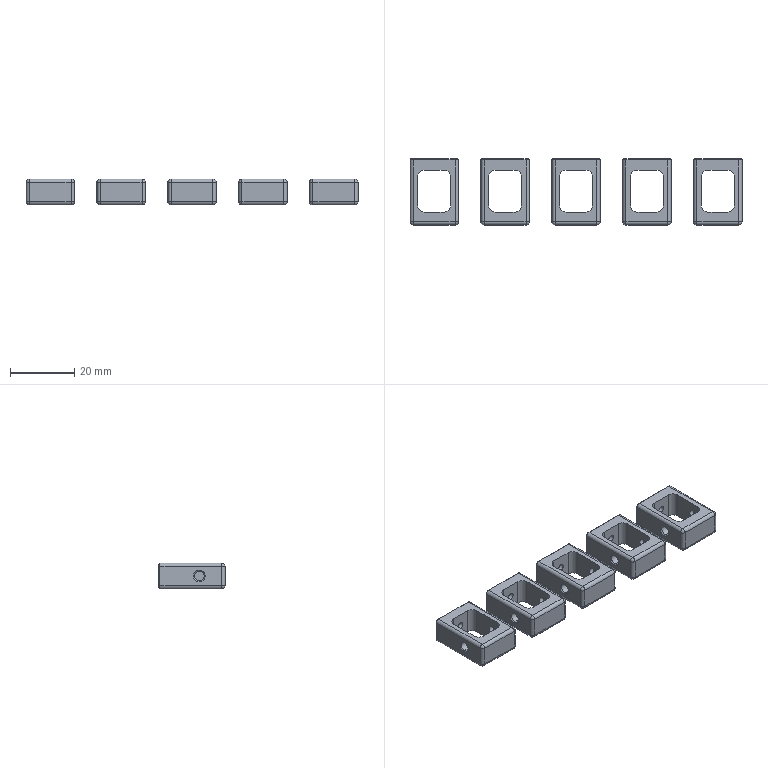NC program | NX | posted with a generic post | part box 103 x 20.5 x 8 mm
Whole program:
N10 G17 G21 G94 G90
(FLOOR_WALL_COPY , TOOL : D80)
N12 T19 M6
N14 G54
N16 G17 G0 G90 X94.5 Y0. S6500 M3
N18 G43 Z30. H19
N20 Z4.
N22 G94 G1 Z1. F1500.
N24 X91.5
N26 X-91.5
N28 X-94.5
N30 Z4.
N32 G0 Z30.
N34 X94.5
N36 Z3.
N38 G1 Z0.
N40 X91.5
N42 X-91.5
N44 X-94.5
N46 Z3.
N48 G0 Z30.
N50 M5
(PLANAR_MILL_COPY_COPY , TOOL : D6A45)
N52 T01 M6
N54 G54
N56 G17 G0 G90 X-47. Y1.02 S9500 M3
N58 G43 Z30. H1
N60 Z0.5
N62 G94 G1 Z-1. F1250.
N64 X-47.7 Y0.616
N66 G3 X-48.2 Y-0.25 R1.
N68 G1 Y-4.75
N70 G3 X-47.1 Y-5.85 R1.1
N72 G1 X-40.9
N74 G3 X-39.8 Y-4.75 R1.1
N76 G1 Y4.25
N78 G3 X-40.9 Y5.35 R1.1
N80 G1 X-47.1
N82 G3 X-48.2 Y4.25 R1.1
N84 G1 Y-0.25
N86 G3 X-47.7 Y-1.116 R1.
N88 G1 X-47. Y-1.52
N90 Z0.5
N92 G0 Z30.
N94 X-25. Y1.02
N96 Z0.5
N98 G1 Z-1.
N100 X-25.7 Y0.616
N102 G3 X-26.2 Y-0.25 R1.
N104 G1 Y-4.75
N106 G3 X-25.1 Y-5.85 R1.1
N108 G1 X-18.9
N110 G3 X-17.8 Y-4.75 R1.1
N112 G1 Y4.25
N114 G3 X-18.9 Y5.35 R1.1
N116 G1 X-25.1
N118 G3 X-26.2 Y4.25 R1.1
N120 G1 Y-0.25
N122 G3 X-25.7 Y-1.116 R1.
N124 G1 X-25. Y-1.52
N126 Z0.5
N128 G0 Z30.
N130 X-3. Y1.02
N132 Z0.5
N134 G1 Z-1.
N136 X-3.7 Y0.616
N138 G3 X-4.2 Y-0.25 R1.
N140 G1 Y-4.75
N142 G3 X-3.1 Y-5.85 R1.1
N144 G1 X3.1
N146 G3 X4.2 Y-4.75 R1.1
N148 G1 Y4.25
N150 G3 X3.1 Y5.35 R1.1
N152 G1 X-3.1
N154 G3 X-4.2 Y4.25 R1.1
N156 G1 Y-0.25
N158 G3 X-3.7 Y-1.116 R1.
N160 G1 X-3. Y-1.52
N162 Z0.5
N164 G0 Z30.
N166 X19. Y1.02
N168 Z0.5
N170 G1 Z-1.
N172 X18.3 Y0.616
N174 G3 X17.8 Y-0.25 R1.
N176 G1 Y-4.75
N178 G3 X18.9 Y-5.85 R1.1
N180 G1 X25.1
N182 G3 X26.2 Y-4.75 R1.1
N184 G1 Y4.25
N186 G3 X25.1 Y5.35 R1.1
N188 G1 X18.9
N190 G3 X17.8 Y4.25 R1.1
N192 G1 Y-0.25
N194 G3 X18.3 Y-1.116 R1.
N196 G1 X19. Y-1.52
N198 Z0.5
N200 G0 Z30.
N202 X47.
N204 Z0.5
N206 G1 Z-1.
N208 X47.7 Y-1.116
N210 G3 X48.2 Y-0.25 R1.
N212 G1 Y4.25
N214 G3 X47.1 Y5.35 R1.1
N216 G1 X40.9
N218 G3 X39.8 Y4.25 R1.1
N220 G1 Y-4.75
N222 G3 X40.9 Y-5.85 R1.1
N224 G1 X47.1
N226 G3 X48.2 Y-4.75 R1.1
N228 G1 Y-0.25
N230 G3 X47.7 Y0.616 R1.
N232 G1 X47. Y1.02
N234 Z0.5
N236 G0 Z30.
N238 M5
(ZLEVEL_PROFILE_1_COPY , TOOL : D4R0.5)
N240 T16 M6
N242 G54
N244 G17 G0 G90 X35.175 Y-12.738 S9500 M3
N246 G43 Z30. H16
N248 Z1.488
N250 G94 G1 Z-0.012 F3000.
N252 X35.682 Y-12.485
N254 G3 X35.903 Y-12.152 R0.4
N256 X35.813 Y-9.95 R10.813
N258 G1 Y9.25
N260 G2 X37.5 Y10.937 R1.687
N262 G1 X50.5
N264 G2 X52.187 Y9.25 R1.687
N266 G1 Y-9.95
N268 X52.109 Y-10.153
N270 X52.09 Y-12.155
N272 X52.133 Y-12.154 Z-0.018
N274 X52.161 Y-12.153 Z-0.024
N276 X52.25 Y-10.153
N278 X52.27 Y-9.95
N280 Y9.25
N282 G3 X50.5 Y11.02 R1.77
N284 G1 X37.5
N286 G3 X35.73 Y9.25 R1.77
N288 G1 Y-9.95
N290 G2 X35.826 Y-12.151 R9.258
N292 G1 X35.785 Y-12.152 Z-0.032
N294 X35.752 Y-12.153 Z-0.039
N296 G3 X35.66 Y-9.95 R7.979
N298 G1 Y9.25
N300 G2 X37.5 Y11.09 R1.84
N302 G1 X50.5
N304 G2 X52.34 Y9.25 R1.84
N306 G1 Y-9.95
N308 X52.223 Y-12.151
N310 X52.264 Y-12.15 Z-0.049
N312 X52.289 Z-0.058
N314 X52.299 Y-11.846
N316 X52.414 Y-9.95
N318 Y9.25
N320 G3 X50.5 Y11.164 R1.914
N322 G1 X37.5
N324 G3 X35.586 Y9.25 R1.914
N326 G1 Y-9.95
N328 G2 X35.684 Y-12.151 R9.178
N330 G1 X35.643 Z-0.07
N332 X35.606 Y-12.15 Z-0.083
N334 G3 X35.509 Y-9.95 R11.176
N336 G1 Y9.25
N338 G2 X37.5 Y11.241 R1.991
N340 G1 X50.5
N342 G2 X52.491 Y9.25 R1.991
N344 G1 Y-9.95
N346 X52.473 Y-10.153
N348 X52.354 Y-12.15
N350 X52.406 Z-0.097
N352 X52.431 Z-0.112
N354 G2 X52.568 Y-9.95 R21.926
N356 G1 Y9.25
N358 G3 X50.5 Y11.318 R2.068
N360 G1 X37.5
N362 G3 X35.432 Y9.25 R2.068
N364 G1 Y-9.95
N366 G2 X35.539 Y-12.15 R11.662
N368 G1 X35.494 Z-0.129
N370 X35.463 Z-0.146
N372 G3 X35.355 Y-9.95 R12.693
N374 G1 Y9.25
N376 G2 X37.5 Y11.395 R2.145
N378 G1 X50.5
N380 G2 X52.645 Y9.25 R2.145
N382 G1 Y-9.95
N384 G3 X52.522 Y-12.15 R18.767
N386 G1 X52.574 Z-0.166
N388 X52.621 Y-12.151 Z-0.186
N390 G2 X52.724 Y-9.95 R19.723
N392 G1 Y9.25
N394 G3 X50.5 Y11.474 R2.224
N396 G1 X37.5
N398 G3 X35.276 Y9.25 R2.224
N400 G1 Y-9.95
N402 G2 X35.374 Y-12.15 R17.072
N404 G1 X35.323 Z-0.21
N406 X35.286 Z-0.233
N408 G3 X35.197 Y-9.95 R17.343
N410 G1 Y9.25
N412 G2 X37.5 Y11.553 R2.303
N414 G1 X50.5
N416 G2 X52.803 Y9.25 R2.303
N418 G1 Y-9.95
N420 G3 X52.716 Y-12.151 R17.692
N422 G1 X52.761 Z-0.259
N424 X52.796 Y-12.15 Z-0.286
N426 G2 X52.881 Y-9.95 R18.852
N428 G1 Y9.25
N430 G3 X50.5 Y11.631 R2.381
N432 G1 X37.5
N434 G3 X35.119 Y9.25 R2.381
N436 G1 Y-9.95
N438 G2 X35.212 Y-12.15 R17.769
N440 G1 X35.16 Z-0.315
N442 X35.13 Z-0.344
N444 G3 X35.044 Y-9.95 R18.76
N446 G1 Y9.25
N448 G2 X37.5 Y11.706 R2.456
N450 G1 X50.5
N452 G2 X52.956 Y9.25 R2.456
N454 G1 Y-9.95
N456 G3 X52.877 Y-12.15 R19.225
N458 G1 X52.92 Y-12.151 Z-0.376
N460 X52.96 Z-0.408
N462 G2 X53.028 Y-9.95 R23.684
N464 G1 Y9.25
N466 G3 X50.5 Y11.778 R2.528
N468 G1 X37.5
N470 G3 X34.972 Y9.25 R2.528
N472 G1 Y-9.95
N474 G2 X35.04 Y-12.15 R23.709
N476 G1 X34.995 Y-12.151 Z-0.443
N478 X34.96 Z-0.477
N480 G3 X34.903 Y-9.95 R26.088
N482 G1 Y9.25
N484 G2 X37.5 Y11.847 R2.597
N486 G1 X50.5
N488 G2 X53.097 Y9.25 R2.597
N490 G1 Y-9.95
N492 G3 X53.04 Y-12.152 R27.115
N494 G1 X53.073 Y-12.151 Z-0.514
N496 X53.1 Y-12.15 Z-0.551
N498 G2 X53.162 Y-9.95 R24.243
N500 G1 Y9.25
N502 G3 X50.5 Y11.912 R2.662
N504 G1 X37.5
N506 G3 X34.838 Y9.25 R2.662
N508 G1 Y-9.95
N510 G2 X34.9 Y-12.151 R24.274
N512 G1 X34.868 Z-0.59
N514 X34.841 Z-0.629
N516 G3 X34.779 Y-9.95 R24.293
N518 G1 Y9.25
N520 G2 X37.5 Y11.971 R2.721
N522 G1 X50.5
N524 G2 X53.221 Y9.25 R2.721
N526 G1 Y-9.95
N528 G3 X53.159 Y-12.151 R24.303
N530 G1 X53.193 Z-0.67
N532 X53.221 Y-12.152 Z-0.711
N534 G2 X53.276 Y-9.95 R30.814
N536 G1 Y9.25
N538 G3 X50.5 Y12.026 R2.776
N540 G1 X37.5
N542 G3 X34.724 Y9.25 R2.776
N544 G1 Y-9.95
N546 G2 X34.779 Y-12.15 R30.37
N548 G1 X34.746 Y-12.151 Z-0.754
N550 X34.728 Z-0.797
N552 G3 X34.675 Y-9.95 R31.84
N554 G1 Y9.25
N556 G2 X37.5 Y12.075 R2.825
N558 G1 X50.5
N560 G2 X53.325 Y9.25 R2.825
N562 G1 Y-9.95
N564 G3 X53.274 Y-12.151 R28.165
N566 G1 X53.299 Z-0.842
N568 X53.317 Z-0.887
N570 G2 X53.369 Y-9.95 R25.497
N572 G1 Y9.25
N574 G3 X50.5 Y12.119 R2.869
N576 G1 X37.5
N578 G3 X34.631 Y9.25 R2.869
N580 G1 Y-9.95
N582 G2 X34.688 Y-12.153 R33.716
N584 G1 X34.663 Y-12.155 Z-0.933
N586 X34.647 Y-12.156 Z-0.979
N588 G3 X34.593 Y-9.95 R49.451
N590 G1 Y9.25
N592 G2 X37.5 Y12.157 R2.907
N594 G1 X50.5
N596 G2 X53.407 Y9.25 R2.907
N598 G1 Y-9.95
N600 G3 X53.362 Y-12.15 R27.233
N602 G1 X53.384 Z-1.026
N604 X53.403 Z-1.074
N606 G2 X53.438 Y-9.95 R31.796
N608 G1 Y9.25
N610 G3 X50.5 Y12.188 R2.938
N612 G1 X37.5
N614 G3 X34.562 Y9.25 R2.938
N616 G1 Y-9.95
N618 G2 X34.608 Y-12.158 R55.585
N620 G1 X34.589 Y-12.16 Z-1.122
N622 X34.572 Y-12.161 Z-1.17
N624 G3 X34.537 Y-9.95 R85.134
N626 G1 Y9.25
N628 G2 X37.5 Y12.213 R2.963
N630 G1 X50.5
N632 G2 X53.463 Y9.25 R2.963
N634 G1 Y-9.95
N636 G3 X53.436 Y-12.152 R39.114
N638 G1 X53.446 Y-12.153 Z-1.212
N640 X53.456 Z-1.253
N642 X53.458 Y-10.717
N644 X53.469 Y-10.435
N646 G2 X53.479 Y-9.95 R3.288
N648 G1 Y9.25
N650 G3 X50.5 Y12.229 R2.979
N652 G1 X37.5
N654 G3 X34.521 Y9.25 R2.979
N656 G1 Y-9.95
N658 G2 X34.55 Y-12.162 R76.351
N660 G1 X34.538 Y-12.163 Z-1.294
N662 X34.531 Z-1.335
N664 X34.516 Y-10.153
N666 X34.509 Y-9.95
N668 Y9.25
N670 G2 X37.5 Y12.241 R2.991
N672 G1 X50.5
N674 G2 X53.491 Y9.25 R2.991
N676 G1 Y-9.95
N678 G3 X53.475 Y-10.717 R24.677
N680 G1 X53.473 Y-12.154
N682 X53.483 Y-12.155 Z-1.376
N684 X53.49 Y-12.156 Z-1.418
N686 X53.492 Y-12.128
N688 X53.496 Y9.273
N690 G3 X53.48 Y9.577 R2.784
N692 X51.216 Y12.161 R2.998
N694 X50.51 Y12.248 R2.956
N696 G1 X37.5
N698 G3 X34.502 Y9.25 R2.998
N700 G1 Y-9.95
N702 X34.511 Y-12.165
N704 X34.505 Y-12.162 Z-1.5
N706 X34.5 Y9.247
N708 G2 X35.313 Y11.3 R2.999
N710 X36.133 Y11.918 R2.897
N712 X36.711 Y12.14 R3.11
N714 X37.518 Y12.248 R3.053
N716 G1 X50.507
N718 G2 X51.524 Y12.069 R2.963
N720 X53.322 Y10.265 R3.012
N722 X53.498 Y9.266 R2.931
N724 G1 X53.495 Y-12.155
N726 G3 X53.695 Y-12.502 R0.4
N728 G1 X54.218 Y-12.804
N730 Z0.
N732 G0 Z3.
N734 X13.176 Y-12.751
N736 Z1.488
N738 G1 Z-0.012
N740 X13.687 Y-12.489
N742 G3 X13.905 Y-12.153 R0.4
N744 X13.813 Y-9.95 R11.978
N746 G1 Y9.25
N748 G2 X15.5 Y10.937 R1.687
N750 G1 X28.5
N752 G2 X30.187 Y9.25 R1.687
N754 G1 Y-9.95
N756 X30.114 Y-10.153
N758 X30.103 Y-12.155
N760 X30.16 Y-12.153 Z-0.024
N762 X30.17 Y-11.846
N764 X30.27 Y-9.95
N766 Y9.25
N768 G3 X28.5 Y11.02 R1.77
N770 G1 X15.5
N772 G3 X13.73 Y9.25 R1.77
N774 G1 Y-9.95
N776 G2 X13.828 Y-12.15 R10.515
N778 G1 X13.781 Z-0.032
N780 X13.776 Z-0.039
N782 G3 X13.66 Y-9.95 R9.336
N784 G1 Y9.25
N786 G2 X15.5 Y11.09 R1.84
N788 G1 X28.5
N790 G2 X30.34 Y9.25 R1.84
N792 G1 Y-9.95
N794 G3 X30.226 Y-12.15 R18.109
N796 G1 X30.26 Z-0.049
N798 X30.281 Z-0.058
N800 G2 X30.414 Y-9.95 R19.419
N802 G1 Y9.25
N804 G3 X28.5 Y11.164 R1.914
N806 G1 X15.5
N808 G3 X13.586 Y9.25 R1.914
N810 G1 Y-9.95
N812 G2 X13.706 Y-12.15 R9.374
N814 G1 X13.643 Z-0.07
N816 X13.618 Z-0.083
N818 G3 X13.509 Y-9.95 R10.828
N820 G1 Y9.25
N822 G2 X15.5 Y11.241 R1.991
N824 G1 X28.5
N826 G2 X30.491 Y9.25 R1.991
N828 G1 Y-9.95
N830 G3 X30.349 Y-12.15 R18.798
N832 G1 X30.406 Z-0.097
N834 X30.431 Z-0.112
N836 G2 X30.568 Y-9.95 R19.096
N838 G1 Y9.25
N840 G3 X28.5 Y11.318 R2.068
N842 G1 X15.5
N844 G3 X13.432 Y9.25 R2.068
N846 G1 Y-9.95
N848 G2 X13.533 Y-12.15 R11.751
N850 G1 X13.494 Z-0.129
N852 X13.46 Z-0.146
N854 G3 X13.355 Y-9.95 R12.417
N856 G1 Y9.25
N858 G2 X15.5 Y11.395 R2.145
N860 G1 X28.5
N862 G2 X30.645 Y9.25 R2.145
N864 G1 Y-9.95
N866 G3 X30.525 Y-12.15 R18.309
N868 G1 X30.574 Y-12.151 Z-0.166
N870 X30.621 Z-0.186
N872 G2 X30.724 Y-9.95 R18.599
N874 G1 Y9.25
N876 G3 X28.5 Y11.474 R2.224
N878 G1 X15.5
N880 G3 X13.276 Y9.25 R2.224
N882 G1 Y-9.95
N884 G2 X13.375 Y-12.15 R15.774
N886 G1 X13.324 Z-0.21
N888 X13.276 Z-0.233
N890 G3 X13.197 Y-9.95 R18.579
N892 G1 Y9.25
N894 G2 X15.5 Y11.553 R2.303
N896 G1 X28.5
N898 G2 X30.803 Y9.25 R2.303
N900 G1 Y-9.95
N902 G3 X30.711 Y-12.151 R19.024
N904 G1 X30.767 Y-12.15 Z-0.259
N906 X30.801 Z-0.286
N908 G2 X30.881 Y-9.95 R18.564
N910 G1 Y9.25
N912 G3 X28.5 Y11.631 R2.381
N914 G1 X15.5
N916 G3 X13.119 Y9.25 R2.381
N918 G1 Y-9.95
N920 G2 X13.206 Y-12.15 R16.93
N922 G1 X13.159 Z-0.315
N924 X13.128 Z-0.344
N926 G3 X13.044 Y-9.95 R17.802
N928 G1 Y9.25
N930 G2 X15.5 Y11.706 R2.456
N932 G1 X28.5
N934 G2 X30.956 Y9.25 R2.456
N936 G1 Y-9.95
N938 G3 X30.877 Y-12.15 R17.906
N940 G1 X30.92 Y-12.151 Z-0.376
N942 X30.96 Z-0.408
N944 G2 X31.028 Y-9.95 R19.425
N946 G1 Y9.25
N948 G3 X28.5 Y11.778 R2.528
N950 G1 X15.5
N952 G3 X12.972 Y9.25 R2.528
N954 G1 Y-9.95
N956 G2 X13.042 Y-12.15 R23.333
N958 G1 X12.995 Z-0.443
N960 X12.967 Z-0.477
N962 G3 X12.903 Y-9.95 R24.397
N964 G1 Y9.25
N966 G2 X15.5 Y11.847 R2.597
N968 G1 X28.5
N970 G2 X31.097 Y9.25 R2.597
N972 G1 Y-9.95
N974 G3 X31.037 Y-12.15 R22.861
N976 G1 X31.069 Z-0.514
N978 X31.1 Z-0.551
N980 G2 X31.162 Y-9.95 R24.207
N982 G1 Y9.25
N984 G3 X28.5 Y11.912 R2.662
N986 G1 X15.5
N988 G3 X12.838 Y9.25 R2.662
N990 G1 Y-9.95
N992 G2 X12.904 Y-12.15 R23.42
N994 G1 X12.868 Y-12.151 Z-0.59
N996 X12.841 Z-0.629
N998 G3 X12.779 Y-9.95 R23.43
N1000 G1 Y9.25
N1002 G2 X15.5 Y11.971 R2.721
N1004 G1 X28.5
N1006 G2 X31.221 Y9.25 R2.721
N1008 G1 Y-9.95
N1010 G3 X31.16 Y-12.151 R24.729
N1012 G1 X31.193 Z-0.67
N1014 X31.222 Z-0.711
N1016 G2 X31.276 Y-9.95 R29.092
N1018 G1 Y9.25
N1020 G3 X28.5 Y12.026 R2.776
N1022 G1 X15.5
N1024 G3 X12.724 Y9.25 R2.776
N1026 G1 Y-9.95
N1028 G2 X12.784 Y-12.15 R25.622
N1030 G1 X12.745 Z-0.754
N1032 X12.726 Z-0.797
N1034 G3 X12.675 Y-9.95 R32.986
N1036 G1 Y9.25
N1038 G2 X15.5 Y12.075 R2.825
N1040 G1 X28.5
N1042 G2 X31.325 Y9.25 R2.825
N1044 G1 Y-9.95
N1046 G3 X31.275 Y-12.152 R33.248
N1048 G1 X31.299 Y-12.151 Z-0.842
N1050 X31.319 Z-0.887
N1052 G2 X31.369 Y-9.95 R28.16
N1054 G1 Y9.25
N1056 G3 X28.5 Y12.119 R2.869
N1058 G1 X15.5
N1060 G3 X12.631 Y9.25 R2.869
N1062 G1 Y-9.95
N1064 G2 X12.684 Y-12.152 R32.786
N1066 G1 X12.663 Y-12.153 Z-0.933
N1068 X12.645 Y-12.154 Z-0.979
N1070 G3 X12.593 Y-9.95 R43.797
N1072 G1 Y9.25
N1074 G2 X15.5 Y12.157 R2.907
N1076 G1 X28.5
N1078 G2 X31.407 Y9.25 R2.907
N1080 G1 Y-9.95
N1082 G3 X31.363 Y-12.15 R27.185
N1084 G1 X31.386 Y-12.152 Z-1.026
N1086 X31.401 Y-12.153 Z-1.074
N1088 G2 X31.438 Y-9.95 R32.305
N1090 G1 Y9.25
N1092 G3 X28.5 Y12.188 R2.938
N1094 G1 X15.5
N1096 G3 X12.562 Y9.25 R2.938
N1098 G1 Y-9.95
N1100 G2 X12.606 Y-12.157 R59.474
N1102 G1 X12.589 Y-12.158 Z-1.122
N1104 X12.572 Y-12.159 Z-1.17
N1106 G3 X12.537 Y-9.95 R87.828
N1108 G1 Y9.25
N1110 G2 X15.5 Y12.213 R2.963
N1112 G1 X28.5
N1114 G2 X31.463 Y9.25 R2.963
N1116 G1 Y-9.95
N1118 G3 X31.436 Y-12.155 R40.13
N1120 G1 X31.446 Z-1.212
N1122 X31.461 Y-12.156 Z-1.253
N1124 G2 X31.479 Y-9.95 R52.452
N1126 G1 Y9.25
N1128 G3 X28.5 Y12.229 R2.979
N1130 G1 X15.5
N1132 G3 X12.521 Y9.25 R2.979
N1134 G1 Y-9.95
N1136 G2 X12.548 Y-12.159 R75.91
N1138 G1 X12.538 Y-12.16 Z-1.294
N1140 X12.53 Y-12.161 Z-1.335
N1142 X12.516 Y-10.153
N1144 X12.509 Y-9.95
N1146 Y9.25
N1148 G2 X15.5 Y12.241 R2.991
N1150 G1 X28.5
N1152 G2 X31.491 Y9.25 R2.991
N1154 G1 Y-9.95
N1156 G3 X31.476 Y-12.157 R76.85
N1158 G1 X31.48 Z-1.376
N1160 X31.491 Y-12.158 Z-1.418
N1162 X31.494 Y-10.153
N1164 X31.497 Y9.272
N1166 G3 X31.48 Y9.574 R2.791
N1168 X29.946 Y11.876 R2.998
N1170 G1 X29.717 Y11.99
N1172 G3 X29.082 Y12.191 R2.998
N1174 X28.5 Y12.248 R2.998
N1176 G1 X15.471
N1178 G3 X13.606 Y11.574 R2.998
N1180 G1 X13.402 Y11.391
N1182 G3 X12.502 Y9.25 R2.998
N1184 G1 Y-9.95
N1186 X12.511 Y-12.162
N1188 X12.505 Y-12.16 Z-1.5
N1190 X12.5 Y9.247
N1192 G2 X13.605 Y11.572 R2.999
N1194 X14.078 Y11.889 R2.738
N1196 X15.35 Y12.242 R2.945
N1198 G1 X15.49 Y12.248
N1200 X28.5
N1202 G2 X29.496 Y12.076 R2.942
N1204 G1 X29.761 Y11.972
N1206 G2 X31.133 Y10.683 R3.033
N1208 X31.498 Y9.26 R3.007
N1210 G1 X31.496 Y-12.128
N1212 X31.495 Y-12.157
N1214 G3 X31.676 Y-12.514 R0.4
N1216 G1 X32.206 Y-12.859
N1218 Z0.
N1220 G0 Z3.
N1222 X-8.825 Y-12.741
N1224 Z1.488
N1226 G1 Z-0.012
N1228 X-8.323 Y-12.489
N1230 G3 X-8.103 Y-12.154 R0.4
N1232 X-8.187 Y-9.95 R11.509
N1234 G1 Y9.25
N1236 G2 X-6.5 Y10.937 R1.687
N1238 G1 X6.5
N1240 G2 X8.187 Y9.25 R1.687
N1242 G1 Y-9.95
N1244 X8.168 Y-10.153
N1246 X8.095 Y-12.155
N1248 X8.134 Y-12.153 Z-0.018
N1250 X8.159 Y-12.152 Z-0.024
N1252 X8.237 Y-10.153
N1254 X8.27 Y-9.95
N1256 Y9.25
N1258 G3 X6.5 Y11.02 R1.77
N1260 G1 X-6.5
N1262 G3 X-8.27 Y9.25 R1.77
N1264 G1 Y-9.95
N1266 G2 X-8.179 Y-12.151 R11.718
N1268 G1 X-8.221 Y-12.15 Z-0.032
N1270 X-8.232 Z-0.039
N1272 G3 X-8.34 Y-9.95 R10.746
N1274 G1 Y9.25
N1276 G2 X-6.5 Y11.09 R1.84
N1278 G1 X6.5
N1280 G2 X8.34 Y9.25 R1.84
N1282 G1 Y-9.95
N1284 X8.298 Y-10.153
N1286 X8.216 Y-12.15
N1288 X8.26 Z-0.049
N1290 X8.274 Z-0.058
N1292 X8.285 Y-11.846
N1294 X8.378 Y-10.153
N1296 X8.414 Y-9.95
N1298 Y9.25
N1300 G3 X6.5 Y11.164 R1.914
N1302 G1 X-6.5
N1304 G3 X-8.414 Y9.25 R1.914
N1306 G1 Y-9.95
N1308 G2 X-8.294 Y-12.15 R9.95
N1310 G1 X-8.357 Z-0.07
N1312 X-8.372 Z-0.083
N1314 G3 X-8.491 Y-9.95 R10.072
N1316 G1 Y9.25
N1318 G2 X-6.5 Y11.241 R1.991
N1320 G1 X6.5
N1322 G2 X8.491 Y9.25 R1.991
N1324 G1 Y-9.95
N1326 G3 X8.348 Y-12.15 R19.167
N1328 G1 X8.405 Z-0.097
N1330 X8.435 Z-0.112
N1332 G2 X8.568 Y-9.95 R20.551
N1334 G1 Y9.25
N1336 G3 X6.5 Y11.318 R2.068
N1338 G1 X-6.5
N1340 G3 X-8.568 Y9.25 R2.068
N1342 G1 Y-9.95
N1344 G2 X-8.465 Y-12.15 R10.922
N1346 G1 X-8.506 Z-0.129
N1348 X-8.538 Z-0.146
N1350 G3 X-8.645 Y-9.95 R11.832
N1352 G1 Y9.25
N1354 G2 X-6.5 Y11.395 R2.145
N1356 G1 X6.5
N1358 G2 X8.645 Y9.25 R2.145
N1360 G1 Y-9.95
N1362 G3 X8.521 Y-12.15 R16.287
N1364 G1 X8.574 Z-0.166
N1366 X8.61 Z-0.186
N1368 G2 X8.724 Y-9.95 R17.188
N1370 G1 Y9.25
N1372 G3 X6.5 Y11.474 R2.224
N1374 G1 X-6.5
N1376 G3 X-8.724 Y9.25 R2.224
N1378 G1 Y-9.95
N1380 G2 X-8.621 Y-12.15 R13.891
N1382 G1 X-8.677 Z-0.21
N1384 X-8.716 Z-0.233
N1386 G3 X-8.803 Y-9.95 R20.219
N1388 G1 Y9.25
N1390 G2 X-6.5 Y11.553 R2.303
N1392 G1 X6.5
N1394 G2 X8.803 Y9.25 R2.303
N1396 G1 Y-9.95
N1398 G3 X8.712 Y-12.15 R22.154
N1400 G1 X8.76 Z-0.259
N1402 X8.798 Z-0.286
N1404 G2 X8.881 Y-9.95 R17.875
N1406 G1 Y9.25
N1408 G3 X6.5 Y11.631 R2.381
N1410 G1 X-6.5
N1412 G3 X-8.881 Y9.25 R2.381
N1414 G1 Y-9.95
N1416 G2 X-8.798 Y-12.15 R17.875
N1418 G1 X-8.841 Z-0.315
N1420 X-8.872 Z-0.344
N1422 G3 X-8.956 Y-9.95 R17.78
N1424 G1 Y9.25
N1426 G2 X-6.5 Y11.706 R2.456
N1428 G1 X6.5
N1430 G2 X8.956 Y9.25 R2.456
N1432 G1 Y-9.95
N1434 G3 X8.872 Y-12.15 R17.78
N1436 G1 X8.92 Z-0.376
N1438 X8.953 Z-0.408
N1440 G2 X9.028 Y-9.95 R21.292
N1442 G1 Y9.25
N1444 G3 X6.5 Y11.778 R2.528
N1446 G1 X-6.5
N1448 G3 X-9.028 Y9.25 R2.528
N1450 G1 Y-9.95
N1452 G2 X-8.953 Y-12.15 R21.292
N1454 G1 X-8.998 Z-0.443
N1456 X-9.041 Z-0.477
N1458 G3 X-9.097 Y-9.95 R25.737
N1460 G1 Y9.25
N1462 G2 X-6.5 Y11.847 R2.597
N1464 G1 X6.5
N1466 G2 X9.097 Y9.25 R2.597
N1468 G1 Y-9.95
N1470 G3 X9.041 Y-12.15 R25.737
N1472 G1 X9.073 Z-0.514
N1474 X9.098 Z-0.551
N1476 G2 X9.162 Y-9.95 R23.081
N1478 G1 Y9.25
N1480 G3 X6.5 Y11.912 R2.662
N1482 G1 X-6.5
N1484 G3 X-9.162 Y9.25 R2.662
N1486 G1 Y-9.95
N1488 G2 X-9.098 Y-12.15 R23.084
N1490 G1 X-9.132 Y-12.151 Z-0.59
N1492 X-9.16 Z-0.629
N1494 G3 X-9.221 Y-9.95 R24.413
N1496 G1 Y9.25
N1498 G2 X-6.5 Y11.971 R2.721
N1500 G1 X6.5
N1502 G2 X9.221 Y9.25 R2.721
N1504 G1 Y-9.95
N1506 G3 X9.16 Y-12.151 R24.402
N1508 G1 X9.193 Z-0.67
N1510 X9.222 Z-0.711
N1512 G2 X9.276 Y-9.95 R30.188
N1514 G1 Y9.25
N1516 G3 X6.5 Y12.026 R2.776
N1518 G1 X-6.5
N1520 G3 X-9.276 Y9.25 R2.776
N1522 G1 Y-9.95
N1524 G2 X-9.222 Y-12.152 R30.24
N1526 G1 X-9.249 Y-12.151 Z-0.754
N1528 X-9.273 Z-0.797
N1530 G3 X-9.325 Y-9.95 R32.017
N1532 G1 Y9.25
N1534 G2 X-6.5 Y12.075 R2.825
N1536 G1 X6.5
N1538 G2 X9.325 Y9.25 R2.825
N1540 G1 Y-9.95
N1542 G3 X9.275 Y-12.151 R29.563
N1544 G1 X9.3 Y-12.15 Z-0.842
N1546 X9.32 Z-0.887
N1548 G2 X9.369 Y-9.95 R27.833
N1550 G1 Y9.25
N1552 G3 X6.5 Y12.119 R2.869
N1554 G1 X-6.5
N1556 G3 X-9.369 Y9.25 R2.869
N1558 G1 Y-9.95
N1560 G2 X-9.316 Y-12.15 R33.813
N1562 G1 X-9.337 Y-12.151 Z-0.933
N1564 X-9.354 Y-12.152 Z-0.979
N1566 G3 X-9.407 Y-9.95 R41.05
N1568 G1 Y9.25
N1570 G2 X-6.5 Y12.157 R2.907
N1572 G1 X6.5
N1574 G2 X9.407 Y9.25 R2.907
N1576 G1 Y-9.95
N1578 G3 X9.362 Y-12.152 R27.311
N1580 G1 X9.383 Y-12.154 Z-1.026
N1582 X9.405 Y-12.156 Z-1.074
N1584 G2 X9.438 Y-9.95 R32.12
N1586 G1 Y9.25
N1588 G3 X6.5 Y12.188 R2.938
N1590 G1 X-6.5
N1592 G3 X-9.438 Y9.25 R2.938
N1594 G1 Y-9.95
N1596 G2 X-9.393 Y-12.155 R76.635
N1598 G1 X-9.411 Y-12.156 Z-1.122
N1600 X-9.428 Y-12.157 Z-1.17
N1602 G3 X-9.463 Y-9.95 R98.832
N1604 G1 Y9.25
N1606 G2 X-6.5 Y12.213 R2.963
N1608 G1 X6.5
N1610 G2 X9.463 Y9.25 R2.963
N1612 G1 Y-9.95
N1614 G3 X9.436 Y-12.157 R39.697
N1616 G1 X9.446 Z-1.212
N1618 X9.458 Z-1.253
N1620 X9.457 Y-11.846
N1622 X9.468 Y-10.153
N1624 X9.479 Y-9.95
N1626 Y9.25
N1628 G3 X6.5 Y12.229 R2.979
N1630 G1 X-6.5
N1632 G3 X-9.479 Y9.25 R2.979
N1634 G1 Y-9.95
N1636 X-9.47 Y-10.153
N1638 X-9.454 Y-12.158
N1640 X-9.462 Y-12.159 Z-1.294
N1642 X-9.472 Z-1.335
N1644 X-9.482 Y-10.153
N1646 X-9.491 Y-9.95
N1648 Y9.25
N1650 G2 X-6.5 Y12.241 R2.991
N1652 G1 X6.5
N1654 G2 X9.491 Y9.25 R2.991
N1656 G1 Y-9.95
N1658 X9.48 Y-10.153
N1660 X9.474 Y-12.159
N1662 X9.482 Z-1.376
N1664 X9.49 Y-12.16 Z-1.418
N1666 X9.492 Y-12.128
N1668 X9.493 Y-10.153
N1670 X9.498 Y-9.95
N1672 Y9.25
N1674 G3 X6.5 Y12.248 R2.998
N1676 G1 X-6.5
N1678 G3 X-9.498 Y9.25 R2.998
N1680 G1 Y-9.95
N1682 X-9.49 Y-12.16
N1684 X-9.495 Y-12.158 Z-1.5
N1686 X-9.497 Y9.324
N1688 G2 X-8.387 Y11.579 R2.989
N1690 G1 X-8.386 Y11.582
N1692 X-8.087 Y11.809
N1694 X-7.668 Y12.011
N1696 X-7.593 Y12.041
N1698 G2 X-6.55 Y12.247 R2.987
N1700 G1 X-6.498 Y12.248
N1702 X6.503
N1704 X6.562 Y12.247
N1706 G2 X7.939 Y11.88 R3.007
N1708 X8.737 Y11.246 R2.745
N1710 X9.338 Y10.215 R2.999
N1712 X9.498 Y9.287 R3.021
N1714 G1 X9.495 Y-12.159
N1716 G3 X9.695 Y-12.506 R0.4
N1718 G1 X10.219 Y-12.809
N1720 Z0.
N1722 G0 Z3.
N1724 X-30.813 Y-12.797
N1726 Z1.488
N1728 G1 Z-0.012
N1730 X-30.306 Y-12.502
N1732 G3 X-30.107 Y-12.155 R0.4
N1734 G1 X-30.114 Y-10.153
N1736 X-30.187 Y-9.95
N1738 Y9.25
N1740 G2 X-28.5 Y10.937 R1.687
N1742 G1 X-15.5
N1744 G2 X-13.813 Y9.25 R1.687
N1746 G1 Y-9.95
N1748 X-13.913 Y-12.155
N1750 X-13.863 Y-12.152 Z-0.018
N1752 X-13.837 Y-12.15 Z-0.024
N1754 X-13.773 Y-10.153
N1756 X-13.73 Y-9.95
N1758 Y9.25
N1760 G3 X-15.5 Y11.02 R1.77
N1762 G1 X-28.5
N1764 G3 X-30.27 Y9.25 R1.77
N1766 G1 Y-9.95
N1768 G2 X-30.178 Y-12.152 R12.211
N1770 G1 X-30.221 Y-12.151 Z-0.032
N1772 X-30.247 Y-12.15 Z-0.039
N1774 G3 X-30.34 Y-9.95 R11.494
N1776 G1 Y9.25
N1778 G2 X-28.5 Y11.09 R1.84
N1780 G1 X-15.5
N1782 G2 X-13.66 Y9.25 R1.84
N1784 G1 Y-9.95
N1786 X-13.705 Y-10.153
N1788 X-13.79 Y-12.15
N1790 X-13.735 Z-0.049
N1792 X-13.727 Z-0.058
N1794 G2 X-13.586 Y-9.95 R19.404
N1796 G1 Y9.25
N1798 G3 X-15.5 Y11.164 R1.914
N1800 G1 X-28.5
N1802 G3 X-30.414 Y9.25 R1.914
N1804 G1 Y-9.95
N1806 G2 X-30.313 Y-12.151 R10.075
N1808 G1 X-30.357 Z-0.07
N1810 X-30.389 Z-0.083
N1812 G3 X-30.491 Y-9.95 R9.024
N1814 G1 Y9.25
N1816 G2 X-28.5 Y11.241 R1.991
N1818 G1 X-15.5
N1820 G2 X-13.509 Y9.25 R1.991
N1822 G1 Y-9.95
N1824 X-13.526 Y-10.153
N1826 X-13.647 Y-12.15
N1828 X-13.596 Z-0.097
N1830 X-13.555 Z-0.112
N1832 G2 X-13.432 Y-9.95 R17.545
N1834 G1 Y9.25
N1836 G3 X-15.5 Y11.318 R2.068
N1838 G1 X-28.5
N1840 G3 X-30.568 Y9.25 R2.068
N1842 G1 Y-9.95
N1844 G2 X-30.461 Y-12.15 R10.15
N1846 G1 X-30.507 Z-0.129
N1848 X-30.538 Z-0.146
N1850 G3 X-30.645 Y-9.95 R12.907
N1852 G1 Y9.25
N1854 G2 X-28.5 Y11.395 R2.145
N1856 G1 X-15.5
N1858 G2 X-13.355 Y9.25 R2.145
N1860 G1 Y-9.95
N1862 G3 X-13.476 Y-12.15 R16.428
N1864 G1 X-13.426 Z-0.166
N1866 X-13.383 Z-0.186
N1868 G2 X-13.276 Y-9.95 R18.66
N1870 G1 Y9.25
N1872 G3 X-15.5 Y11.474 R2.224
N1874 G1 X-28.5
N1876 G3 X-30.724 Y9.25 R2.224
N1878 G1 Y-9.95
N1880 G2 X-30.616 Y-12.15 R19.048
N1882 G1 X-30.678 Z-0.21
N1884 X-30.705 Z-0.233
N1886 G3 X-30.803 Y-9.95 R20.974
N1888 G1 Y9.25
N1890 G2 X-28.5 Y11.553 R2.303
N1892 G1 X-15.5
N1894 G2 X-13.197 Y9.25 R2.303
N1896 G1 Y-9.95
N1898 G3 X-13.276 Y-12.15 R18.579
N1900 G1 X-13.238 Z-0.259
N1902 X-13.206 Z-0.286
N1904 G2 X-13.119 Y-9.95 R16.93
N1906 G1 Y9.25
N1908 G3 X-15.5 Y11.631 R2.381
N1910 G1 X-28.5
N1912 G3 X-30.881 Y9.25 R2.381
N1914 G1 Y-9.95
N1916 G2 X-30.801 Y-12.15 R18.564
N1918 G1 X-30.841 Z-0.315
N1920 X-30.877 Z-0.344
N1922 G3 X-30.956 Y-9.95 R17.906
N1924 G1 Y9.25
N1926 G2 X-28.5 Y11.706 R2.456
N1928 G1 X-15.5
N1930 G2 X-13.044 Y9.25 R2.456
N1932 G1 Y-9.95
N1934 G3 X-13.128 Y-12.15 R17.802
N1936 G1 X-13.08 Z-0.376
N1938 X-13.042 Z-0.408
N1940 G2 X-12.972 Y-9.95 R23.333
N1942 G1 Y9.25
N1944 G3 X-15.5 Y11.778 R2.528
N1946 G1 X-28.5
N1948 G3 X-31.028 Y9.25 R2.528
N1950 G1 Y-9.95
N1952 G2 X-30.96 Y-12.151 R19.425
N1954 G1 X-30.999 Z-0.443
N1956 X-31.037 Y-12.15 Z-0.477
N1958 G3 X-31.097 Y-9.95 R22.861
N1960 G1 Y9.25
N1962 G2 X-28.5 Y11.847 R2.597
N1964 G1 X-15.5
N1966 G2 X-12.903 Y9.25 R2.597
N1968 G1 Y-9.95
N1970 G3 X-12.967 Y-12.15 R24.397
N1972 G1 X-12.927 Z-0.514
N1974 X-12.904 Z-0.551
N1976 G2 X-12.838 Y-9.95 R23.42
N1978 G1 Y9.25
N1980 G3 X-15.5 Y11.912 R2.662
N1982 G1 X-28.5
N1984 G3 X-31.162 Y9.25 R2.662
N1986 G1 Y-9.95
N1988 G2 X-31.1 Y-12.15 R24.209
N1990 G1 X-31.132 Y-12.151 Z-0.59
N1992 X-31.16 Z-0.629
N1994 G3 X-31.221 Y-9.95 R24.736
N1996 G1 Y9.25
N1998 G2 X-28.5 Y11.971 R2.721
N2000 G1 X-15.5
N2002 G2 X-12.779 Y9.25 R2.721
N2004 G1 Y-9.95
N2006 G3 X-12.841 Y-12.151 R23.43
N2008 G1 X-12.807 Y-12.15 Z-0.67
N2010 X-12.784 Z-0.711
N2012 G2 X-12.724 Y-9.95 R25.622
N2014 G1 Y9.25
N2016 G3 X-15.5 Y12.026 R2.776
N2018 G1 X-28.5
N2020 G3 X-31.276 Y9.25 R2.776
N2022 G1 Y-9.95
N2024 G2 X-31.222 Y-12.152 R29.106
N2026 G1 X-31.248 Z-0.754
N2028 X-31.275 Z-0.797
N2030 G3 X-31.325 Y-9.95 R33.53
N2032 G1 Y9.25
N2034 G2 X-28.5 Y12.075 R2.825
N2036 G1 X-15.5
N2038 G2 X-12.675 Y9.25 R2.825
N2040 G1 Y-9.95
N2042 G3 X-12.726 Y-12.15 R32.804
N2044 G1 X-12.7 Y-12.151 Z-0.842
N2046 X-12.68 Y-12.152 Z-0.887
N2048 G2 X-12.631 Y-9.95 R27.974
N2050 G1 Y9.25
N2052 G3 X-15.5 Y12.119 R2.869
N2054 G1 X-28.5
N2056 G3 X-31.369 Y9.25 R2.869
N2058 G1 Y-9.95
N2060 G2 X-31.316 Y-12.151 R34.661
N2062 G1 X-31.337 Y-12.15 Z-0.933
N2064 X-31.355 Z-0.979
N2066 G3 X-31.407 Y-9.95 R42.325
N2068 G1 Y9.25
N2070 G2 X-28.5 Y12.157 R2.907
N2072 G1 X-15.5
N2074 G2 X-12.593 Y9.25 R2.907
N2076 G1 Y-9.95
N2078 G3 X-12.637 Y-12.155 R28.211
N2080 G1 X-12.616 Y-12.156 Z-1.026
N2082 X-12.597 Z-1.074
N2084 G2 X-12.562 Y-9.95 R32.34
N2086 G1 Y9.25
N2088 G3 X-15.5 Y12.188 R2.938
N2090 G1 X-28.5
N2092 G3 X-31.438 Y9.25 R2.938
N2094 G1 Y-9.95
N2096 G2 X-31.392 Y-12.152 R56.529
N2098 G1 X-31.411 Y-12.153 Z-1.122
N2100 X-31.428 Y-12.154 Z-1.17
N2102 G3 X-31.463 Y-9.95 R90.183
N2104 G1 Y9.25
N2106 G2 X-28.5 Y12.213 R2.963
N2108 G1 X-15.5
N2110 G2 X-12.537 Y9.25 R2.963
N2112 G1 Y-9.95
N2114 G3 X-12.565 Y-12.159 R39.861
N2116 G1 X-12.554 Z-1.212
N2118 X-12.545 Z-1.253
N2120 X-12.542 Y-10.717
N2122 X-12.531 Y-10.435
N2124 G2 X-12.521 Y-9.95 R3.235
N2126 G1 Y9.25
N2128 G3 X-15.5 Y12.229 R2.979
N2130 G1 X-28.5
N2132 G3 X-31.479 Y9.25 R2.979
N2134 G1 Y-9.95
N2136 X-31.471 Y-10.153
N2138 X-31.462 Y-10.999
N2140 X-31.455 Y-11.995
N2142 X-31.448 Y-12.155
N2144 X-31.462 Y-12.156 Z-1.294
N2146 X-31.469 Y-12.157 Z-1.335
N2148 X-31.476 Y-11.282
N2150 X-31.483 Y-10.153
N2152 X-31.491 Y-9.95
N2154 Y9.25
N2156 G2 X-28.5 Y12.241 R2.991
N2158 G1 X-15.5
N2160 G2 X-12.509 Y9.25 R2.991
N2162 G1 Y-9.95
N2164 G3 X-12.525 Y-10.717 R24.766
N2166 G1 X-12.527 Y-12.161
N2168 X-12.519 Y-12.162 Z-1.376
N2170 X-12.51 Z-1.418
N2172 X-12.508 Y-12.128
N2174 X-12.507 Y-10.153
N2176 X-12.502 Y-9.95
N2178 Y9.25
N2180 G3 X-14.882 Y12.183 R2.998
N2182 X-15.49 Y12.248 R2.95
N2184 G1 X-28.5
N2186 G3 X-31.498 Y9.25 R2.998
N2188 G1 Y-9.95
N2190 X-31.495 Y-10.153
N2192 X-31.491 Y-12.128
N2194 X-31.489 Y-12.158
N2196 X-31.495 Y-12.157 Z-1.5
N2198 X-31.498 Y9.267
N2200 G2 X-30.825 Y11.135 R2.931
N2202 X-30.426 Y11.547 R2.509
N2204 G1 X-30.346 Y11.612
N2206 G2 X-29.946 Y11.876 R2.38
N2208 G1 X-29.673 Y12.011
N2210 G2 X-29.047 Y12.197 R2.783
N2212 X-28.5 Y12.248 R3.232
N2214 G1 X-15.49
N2216 G2 X-14.06 Y11.879 R3.014
N2218 X-13.588 Y11.559 R2.811
N2220 X-12.891 Y10.731 R3.118
N2222 G1 X-12.723 Y10.379
N2224 X-12.692 Y10.3
N2226 G2 X-12.547 Y9.767 R2.477
N2228 X-12.502 Y9.287 R3.255
N2230 G1 X-12.505 Y-12.161
N2232 G3 X-12.305 Y-12.507 R0.4
N2234 G1 X-11.783 Y-12.809
N2236 Z0.
N2238 G0 Z3.
N2240 X-52.79 Y-12.831
N2242 Z1.488
N2244 G1 Z-0.012
N2246 X-52.25 Y-12.501
N2248 G3 X-52.059 Y-12.15 R0.4
N2250 G1 X-52.109 Y-10.153
N2252 X-52.187 Y-9.95
N2254 Y9.25
N2256 G2 X-50.5 Y10.937 R1.687
N2258 G1 X-37.5
N2260 G2 X-35.813 Y9.25 R1.687
N2262 G1 Y-9.95
N2264 X-35.849 Y-10.153
N2266 X-35.907 Y-11.846
N2268 X-35.91 Y-12.153
N2270 X-35.863 Y-12.151 Z-0.018
N2272 X-35.845 Y-12.15 Z-0.024
N2274 X-35.781 Y-10.153
N2276 X-35.73 Y-9.95
N2278 Y9.25
N2280 G3 X-37.5 Y11.02 R1.77
N2282 G1 X-50.5
N2284 G3 X-52.27 Y9.25 R1.77
N2286 G1 Y-9.95
N2288 G2 X-52.145 Y-12.15 R14.513
N2290 G1 X-52.215 Z-0.032
N2292 X-52.243 Z-0.039
N2294 G3 X-52.34 Y-9.95 R11.799
N2296 G1 Y9.25
N2298 G2 X-50.5 Y11.09 R1.84
N2300 G1 X-37.5
N2302 G2 X-35.66 Y9.25 R1.84
N2304 G1 Y-9.95
N2306 X-35.703 Y-10.153
N2308 X-35.794 Y-12.15
N2310 X-35.74 Z-0.049
N2312 X-35.727 Z-0.058
N2314 G2 X-35.586 Y-9.95 R25.754
N2316 G1 Y9.25
N2318 G3 X-37.5 Y11.164 R1.914
N2320 G1 X-50.5
N2322 G3 X-52.414 Y9.25 R1.914
N2324 G1 Y-9.95
N2326 G2 X-52.316 Y-12.15 R10.975
N2328 G1 X-52.357 Y-12.151 Z-0.07
N2330 X-52.394 Y-12.152 Z-0.083
N2332 G3 X-52.491 Y-9.95 R10.031
N2334 G1 Y9.25
N2336 G2 X-50.5 Y11.241 R1.991
N2338 G1 X-37.5
N2340 G2 X-35.509 Y9.25 R1.991
N2342 G1 Y-9.95
N2344 G3 X-35.642 Y-12.15 R24.332
N2346 G1 X-35.595 Z-0.097
N2348 X-35.558 Z-0.112
N2350 G2 X-35.432 Y-9.95 R16.369
N2352 G1 Y9.25
N2354 G3 X-37.5 Y11.318 R2.068
N2356 G1 X-50.5
N2358 G3 X-52.568 Y9.25 R2.068
N2360 G1 Y-9.95
N2362 G2 X-52.463 Y-12.151 R10.22
N2364 G1 X-52.507 Y-12.15 Z-0.129
N2366 X-52.541 Z-0.146
N2368 G3 X-52.645 Y-9.95 R12.053
N2370 G1 Y9.25
N2372 G2 X-50.5 Y11.395 R2.145
N2374 G1 X-37.5
N2376 G2 X-35.355 Y9.25 R2.145
N2378 G1 Y-9.95
N2380 G3 X-35.476 Y-12.15 R15.899
N2382 G1 X-35.426 Z-0.166
N2384 X-35.38 Z-0.186
N2386 G2 X-35.276 Y-9.95 R18.924
N2388 G1 Y9.25
N2390 G3 X-37.5 Y11.474 R2.224
N2392 G1 X-50.5
N2394 G3 X-52.724 Y9.25 R2.224
N2396 G1 Y-9.95
N2398 G2 X-52.627 Y-12.151 R16.637
N2400 G1 X-52.677 Z-0.21
N2402 X-52.716 Z-0.233
N2404 G3 X-52.803 Y-9.95 R17.677
N2406 G1 Y9.25
N2408 G2 X-50.5 Y11.553 R2.303
N2410 G1 X-37.5
N2412 G2 X-35.197 Y9.25 R2.303
N2414 G1 Y-9.95
N2416 G3 X-35.286 Y-12.15 R17.35
N2418 G1 X-35.238 Z-0.259
N2420 X-35.212 Z-0.286
N2422 G2 X-35.119 Y-9.95 R17.769
N2424 G1 Y9.25
N2426 G3 X-37.5 Y11.631 R2.381
N2428 G1 X-50.5
N2430 G3 X-52.881 Y9.25 R2.381
N2432 G1 Y-9.95
N2434 G2 X-52.796 Y-12.15 R18.849
N2436 G1 X-52.841 Z-0.315
N2438 X-52.877 Z-0.344
N2440 G3 X-52.956 Y-9.95 R19.225
N2442 G1 Y9.25
N2444 G2 X-50.5 Y11.706 R2.456
N2446 G1 X-37.5
N2448 G2 X-35.044 Y9.25 R2.456
N2450 G1 Y-9.95
N2452 G3 X-35.13 Y-12.15 R18.76
N2454 G1 X-35.08 Z-0.376
N2456 X-35.04 Z-0.408
N2458 G2 X-34.972 Y-9.95 R23.709
N2460 G1 Y9.25
N2462 G3 X-37.5 Y11.778 R2.528
N2464 G1 X-50.5
N2466 G3 X-53.028 Y9.25 R2.528
N2468 G1 Y-9.95
N2470 G2 X-52.96 Y-12.151 R23.684
N2472 G1 X-52.999 Z-0.443
N2474 X-53.04 Y-12.152 Z-0.477
N2476 G3 X-53.097 Y-9.95 R26.941
N2478 G1 Y9.25
N2480 G2 X-50.5 Y11.847 R2.597
N2482 G1 X-37.5
N2484 G2 X-34.903 Y9.25 R2.597
N2486 G1 Y-9.95
N2488 G3 X-34.96 Y-12.151 R26.088
N2490 G1 X-34.93 Z-0.514
N2492 X-34.9 Z-0.551
N2494 G2 X-34.838 Y-9.95 R24.274
N2496 G1 Y9.25
N2498 G3 X-37.5 Y11.912 R2.662
N2500 G1 X-50.5
N2502 G3 X-53.162 Y9.25 R2.662
N2504 G1 Y-9.95
N2506 G2 X-53.1 Y-12.15 R24.243
N2508 G1 X-53.132 Z-0.59
N2510 X-53.159 Y-12.151 Z-0.629
N2512 G3 X-53.221 Y-9.95 R24.309
N2514 G1 Y9.25
N2516 G2 X-50.5 Y11.971 R2.721
N2518 G1 X-37.5
N2520 G2 X-34.779 Y9.25 R2.721
N2522 G1 Y-9.95
N2524 G3 X-34.841 Y-12.151 R24.293
N2526 G1 X-34.807 Y-12.15 Z-0.67
N2528 X-34.779 Z-0.711
N2530 G2 X-34.724 Y-9.95 R30.37
N2532 G1 Y9.25
N2534 G3 X-37.5 Y12.026 R2.776
N2536 G1 X-50.5
N2538 G3 X-53.276 Y9.25 R2.776
N2540 G1 Y-9.95
N2542 G2 X-53.221 Y-12.152 R30.832
N2544 G1 X-53.249 Z-0.754
N2546 X-53.272 Y-12.151 Z-0.797
N2548 G3 X-53.325 Y-9.95 R30.716
N2550 G1 Y9.25
N2552 G2 X-50.5 Y12.075 R2.825
N2554 G1 X-37.5
N2556 G2 X-34.675 Y9.25 R2.825
N2558 G1 Y-9.95
N2560 G3 X-34.726 Y-12.151 R29.111
N2562 G1 X-34.701 Y-12.153 Z-0.842
N2564 X-34.682 Y-12.154 Z-0.887
N2566 G2 X-34.631 Y-9.95 R25.64
N2568 G1 Y9.25
N2570 G3 X-37.5 Y12.119 R2.869
N2572 G1 X-50.5
N2574 G3 X-53.369 Y9.25 R2.869
N2576 G1 Y-9.95
N2578 G2 X-53.312 Y-12.151 R32.482
N2580 G1 X-53.337 Z-0.933
N2582 X-53.353 Z-0.979
N2584 G3 X-53.407 Y-9.95 R44.733
N2586 G1 Y9.25
N2588 G2 X-50.5 Y12.157 R2.907
N2590 G1 X-37.5
N2592 G2 X-34.593 Y9.25 R2.907
N2594 G1 Y-9.95
N2596 G3 X-34.638 Y-12.157 R27.476
N2598 G1 X-34.616 Y-12.158 Z-1.026
N2600 X-34.6 Y-12.159 Z-1.074
N2602 G2 X-34.562 Y-9.95 R31.
N2604 G1 Y9.25
N2606 G3 X-37.5 Y12.188 R2.938
N2608 G1 X-50.5
N2610 G3 X-53.438 Y9.25 R2.938
N2612 G1 Y-9.95
N2614 G2 X-53.395 Y-12.15 R54.144
N2616 G1 X-53.413 Y-12.151 Z-1.122
N2618 X-53.428 Y-12.152 Z-1.17
N2620 G3 X-53.463 Y-9.95 R83.256
N2622 G1 Y9.25
N2624 G2 X-50.5 Y12.213 R2.963
N2626 G1 X-37.5
N2628 G2 X-34.537 Y9.25 R2.963
N2630 G1 Y-9.95
N2632 G3 X-34.564 Y-12.161 R40.729
N2634 G1 X-34.554 Y-12.164 Z-1.212
N2636 X-34.541 Y-12.167 Z-1.253
N2638 G2 X-34.521 Y-9.95 R43.821
N2640 G1 Y9.25
N2642 G3 X-37.5 Y12.229 R2.979
N2644 G1 X-50.5
N2646 G3 X-53.479 Y9.25 R2.979
N2648 G1 Y-9.95
N2650 X-53.468 Y-10.153
N2652 X-53.452 Y-12.153
N2654 X-53.462 Y-12.154 Z-1.294
N2656 X-53.471 Z-1.335
N2658 X-53.481 Y-10.153
N2660 X-53.491 Y-9.95
N2662 Y9.25
N2664 G2 X-50.5 Y12.241 R2.991
N2666 G1 X-37.5
N2668 G2 X-34.509 Y9.25 R2.991
N2670 G1 Y-9.95
N2672 X-34.518 Y-10.153
N2674 X-34.528 Y-11.846
N2676 X-34.525 Y-12.167
N2678 X-34.518 Y-12.166 Z-1.376
N2680 X-34.51 Y-12.165 Z-1.418
N2682 X-34.507 Y-10.153
N2684 X-34.502 Y-9.95
N2686 Y9.25
N2688 G3 X-37.5 Y12.248 R2.998
N2690 G1 X-50.5
N2692 G3 X-53.498 Y9.25 R2.998
N2694 G1 Y-9.95
N2696 X-53.49 Y-12.156
N2698 X-53.495 Y-12.155 Z-1.5
N2700 X-53.498 Y9.287
N2702 G2 X-52.392 Y11.575 R2.988
N2704 G1 X-52.386 Y11.582
N2706 X-52.075 Y11.816
N2708 G2 X-51.315 Y12.135 R4.006
N2710 X-50.851 Y12.227 R2.683
N2712 G1 Y12.226
N2714 X-50.568 Y12.246
N2716 X-50.51 Y12.248
N2718 X-37.49
N2720 X-37.44 Y12.247
N2722 G2 X-36.06 Y11.879 R3.08
N2724 X-35.191 Y11.152 R2.814
N2726 X-34.877 Y10.7 R2.554
N2728 G1 X-34.72 Y10.372
N2730 X-34.701 Y10.324
N2732 G2 X-34.547 Y9.767 R2.585
N2734 X-34.502 Y9.287 R3.272
N2736 G1 X-34.505 Y-12.163
N2738 G3 X-34.305 Y-12.509 R0.4
N2740 G1 X-33.783 Y-12.811
N2742 Z0.
N2744 G0 Z30.
N2746 M5
N2748 M2